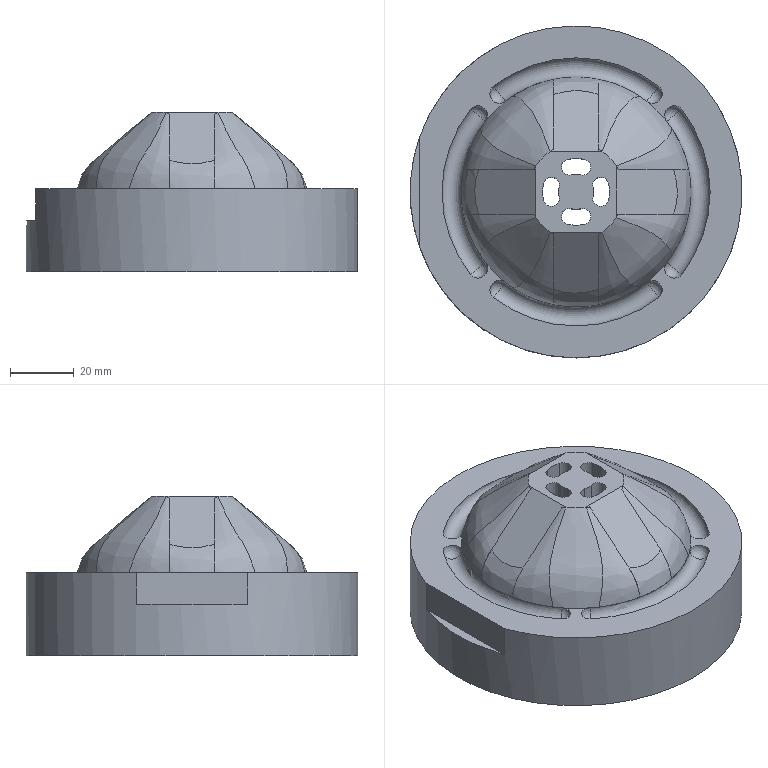CAM job | NX | 3-axis milling | part box 104 x 104 x 49.86 mm | stock box 104 x 104 x 49.86 mm
Tools:
number,name,description,diameter,corner_radius,flute_length,length,flutes
0,D20R0.8,Milling Tool-5 Parameters,20.0,0.8,50.0,75.0,2
0,B,Milling Tool-Ball Mill,6.0,3.0,50.0,75.0,2
0,B12,Milling Tool-Ball Mill,12.0,6.0,50.0,75.0,2
0,D10,Milling Tool-5 Parameters,10.0,0.0,50.0,75.0,2
Operations:
program,operation,operation_type,tool,method,geometry_group,spindle_rpm,surface_speed,feed_per_tooth,feed_cut,feed_plunge,cut_length_mm,path_length_mm,cut_time_min,machine_time_min
NC_PROGRAM,CAVITY_MILL,CavityMilling,D20R0.8,METHOD,WORKPIECE,2992.0,282.0,0.4178,2500.0,50.0,36733.287,39076.28,15.022,15.391
NC_PROGRAM,FACE_MILLING,FaceMilling,D20R0.8,METHOD,WORKPIECE,3000.0,282.0,0.4167,2500.0,50.0,499.179,670.457,0.221,0.2381
NC_PROGRAM,PLANAR_MILL,PlanarMilling,B,METHOD,WORKPIECE,2122.0,40.0,0.185,785.2,100.0,2969.132,3450.902,3.781,3.829
NC_PROGRAM,PLANAR_MILL_COPY,PlanarMilling,B,METHOD,WORKPIECE,2122.0,40.0,0.185,785.2,100.0,230.926,610.326,0.2941,0.332
NC_PROGRAM,ZLEVEL_PROFILE,ZLevelMilling,B12,METHOD,WORKPIECE,3000.0,282.0,0.4167,2500.0,80.0,15435.445,16075.928,6.184,6.248
NC_PROGRAM,ZLEVEL_PROFILE_COPY,ZLevelMilling,B12,METHOD,WORKPIECE,3000.0,282.0,0.4167,2500.0,80.0,23010.509,23073.97,9.206,9.212
NC_PROGRAM,ZLEVEL_PROFILE_COPY_COPY,ZLevelMilling,D10,METHOD,WORKPIECE,3000.0,282.0,0.4167,2500.0,80.0,108.444,301.885,0.0453,0.0647
NC_PROGRAM,PLUNGE_MILLING,PlungeMilling,D20R0.8,METHOD,WORKPIECE,1000.0,94.0,0.125,250.0,100.0,1197.297,2288.09,4.789,4.898